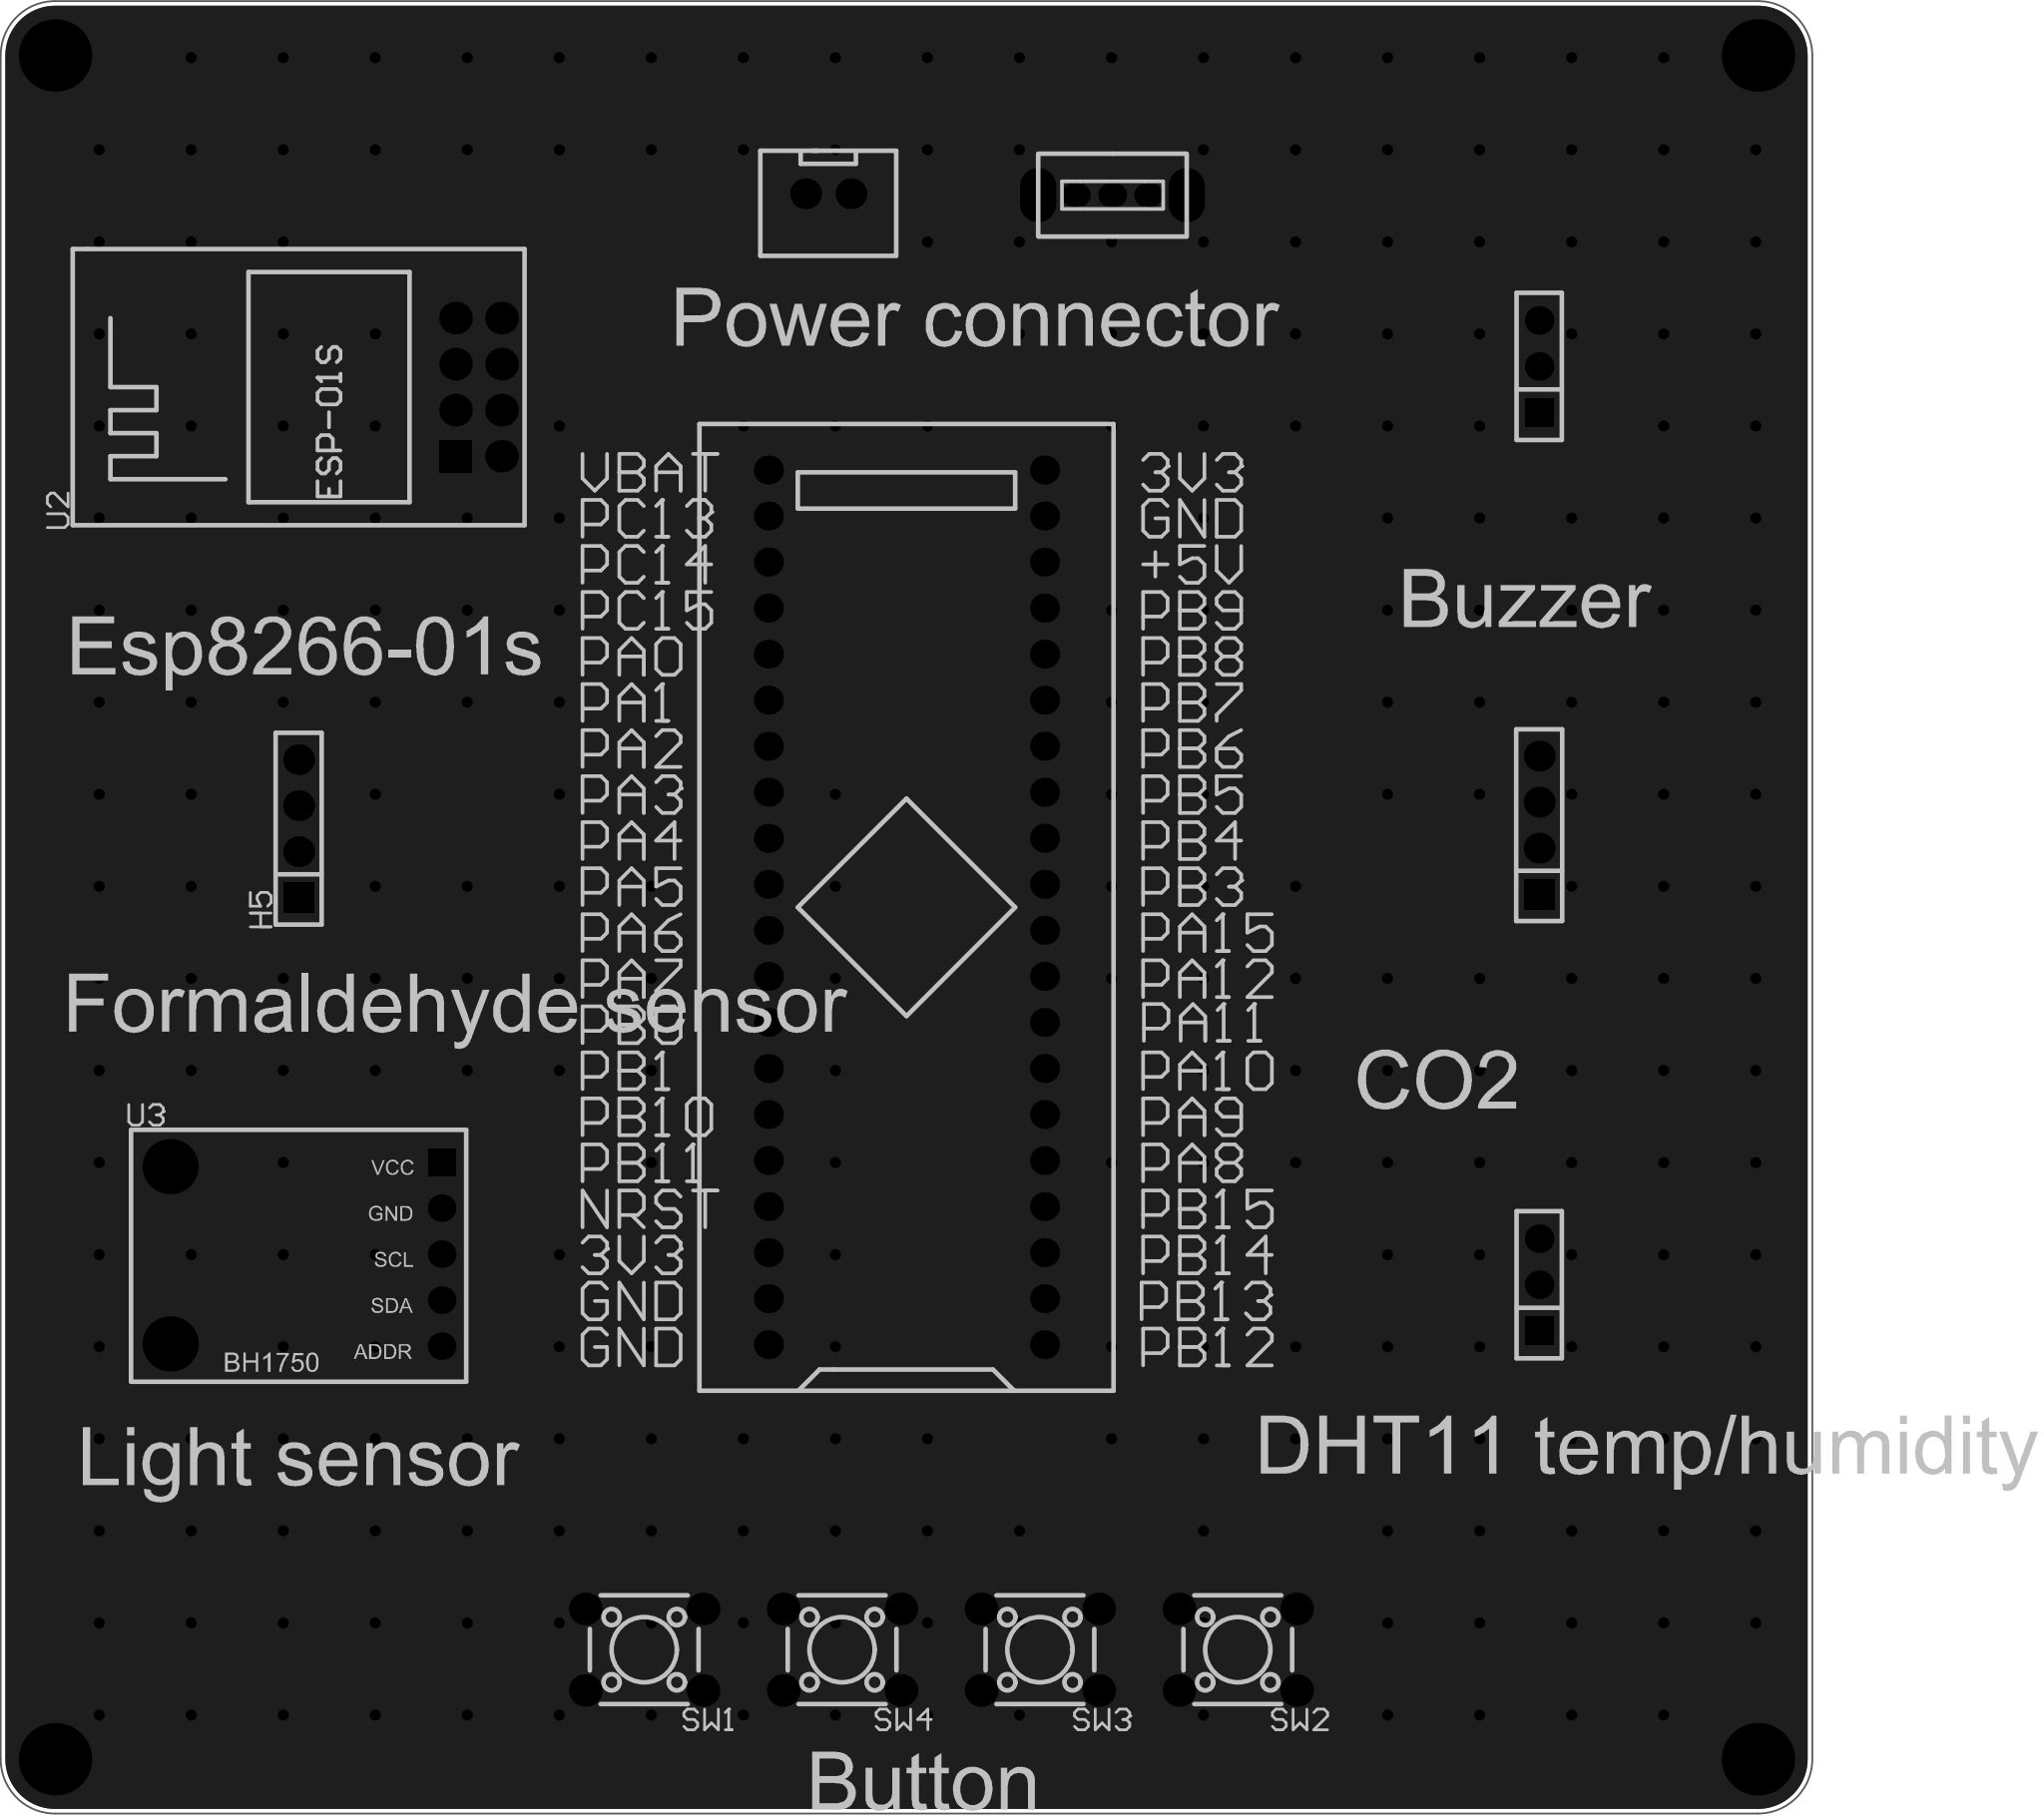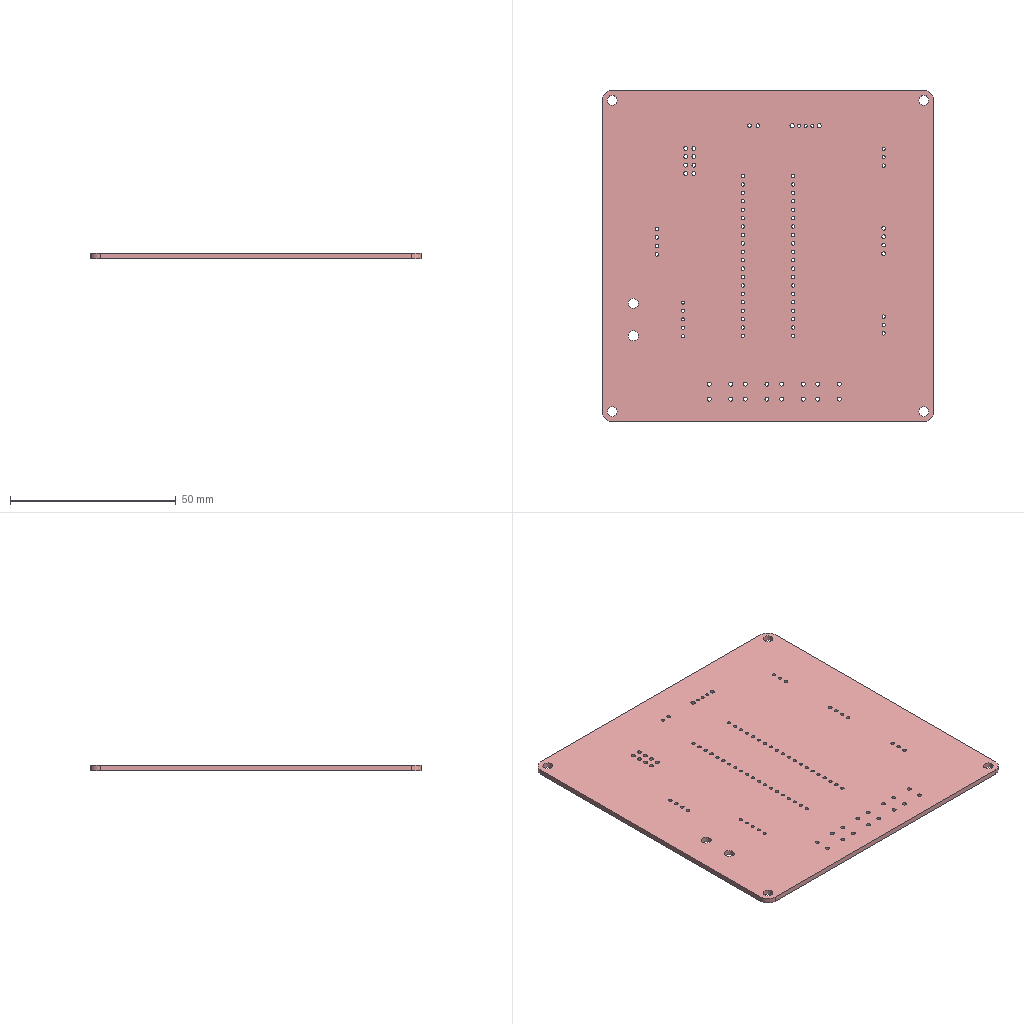Circuit board layout | Altium Designer | box 100 x 100 x 1.6 mm
Layer stack:
# Altium Designer layer stack of  (unit mm; dielectric type: 0 none, 1 core, 2 prepreg, 3 surface material)
index,name,kind,layer,copper_thickness_mm,dielectric_type,dielectric_thickness_mm,dielectric_material,dielectric_constant
0,Top Paste Mask Layer,other,,,,,,
1,Top Silkscreen Layer,other,,,,,,
2,Top Solder Mask Layer,dielectric,,,3,0.01,,3.3
3,Top Layer,copper,Top Layer,0.035,,,,
4,Dielectric1,dielectric,,,3,1.51,FR4,4.5
5,Bottom Layer,copper,Bottom Layer,0.035,,,,
6,Bottom Solder Mask Layer,dielectric,,,3,0.01,,3.3
7,Bottom Silkscreen Layer,other,,,,,,
8,Bottom Paste Mask Layer,other,,,,,,
# drill layer pairs: low layer,high layer
drill_pair,Top Layer,Bottom Layer
Part placement:
Designator,Comment,Layer,Footprint,Center-X(mm),Center-Y(mm),Rotation
U1,STM32F103C8T6-Card,TopLayer,CONN-TH_L53.3-W22.9_STM32F103C8T6-CARD,141.351,130.937,90
SW1,,TopLayer,SW-TH_4P-L6.0-W6.0-P4.50-LS6.5,126.873,89.979,180
SW2,,TopLayer,SW-TH_4P-L6.0-W6.0-P4.50-LS6.5,159.639,89.979,180
SW3,,TopLayer,SW-TH_4P-L6.0-W6.0-P4.50-LS6.5,148.717,89.979,180
SW4,,TopLayer,SW-TH_4P-L6.0-W6.0-P4.50-LS6.5,137.795,89.979,180
CN4,XH2.54*2P_Through-hole,TopLayer,CONN-TH_2P-P2.50-XH2.54-2P,137.033,170.307,0
SW5,,TopLayer,拨动开关,152.72,170.232,180
H1,,TopLayer,HDR-TH_3P-P2.54-V-F,176.276,160.782,90
H3,,TopLayer,HDR-TH_3P-P2.54-V-F,176.276,110.113,90
H4,,TopLayer,HDR-TH_4P-P2.54-V-F,176.276,135.47,90
H5,,TopLayer,HDR-TH_4P-P2.54-V-F,107.798,135.275,90
U2,ESP-01S,TopLayer,WIFIM-TH_ESP-01S,117.729,159.639,90
U3,,TopLayer,BH1750光照传感器,108.2,111.805,0
Pad and via stacks:
# Altium Designer via and pad stacks of  (unit mm). Each distinct definition once, with the count of objects using it.
# via: kind,start_layer,end_layer,hole_mm,diameter_mm,mode(0 simple;1 top-mid-bottom;2 full stack),diameter_per_layer,count,example_net
# pad: kind,layer,hole_mm,hole_type(0 round;1 square;2 slot),plating,top_size,top_shape(1 round;2 rect;3 octagon;9 rounded rect),mid_size,bottom_size,mode,footprint,size_per_layer,count,example
pad,Multi-Layer,3,0,plated,4x4,1,4x4,4x4,0,,,4,1
pad,Multi-Layer,1,0,plated,1.6x1.6,1,1.6x1.6,1.6x1.6,0,CONN-TH_L53.3-W22.9_STM32F103C8T6-CARD,,40,U1.1
pad,Multi-Layer,1.2,0,plated,1.8x1.8,1,1.8x1.8,1.8x1.8,0,SW-TH_4P-L6.0-W6.0-P4.50-LS6.5,,16,SW1.1
pad,Multi-Layer,1.05,0,plated,1.7x1.7,1,1.7x1.7,1.7x1.7,0,CONN-TH_2P-P2.50-XH2.54-2P,,2,CN4.2
pad,Multi-Layer,0.8992,0,plated,1.6x1.3,1,1.6x1.3,1.6x1.3,0,\u00B2\u00A6\u00B6\u00AF\u00BF\u00AA\u00B9\u00D8,,3,SW5.1
pad,Multi-Layer,1.3,0,plated,3x1.999,1,3x1.999,3x1.999,0,\u00B2\u00A6\u00B6\u00AF\u00BF\u00AA\u00B9\u00D8,,2,SW5.4
pad,Multi-Layer,1.02,0,plated,1.575x1.575,1,1.575x1.575,1.575x1.575,0,HDR-TH_3P-P2.54-V-F,,4,H1.3
pad,Multi-Layer,1.02,0,plated,1.575x1.575,2,1.575x1.575,1.575x1.575,0,HDR-TH_3P-P2.54-V-F,,2,H1.1
pad,Multi-Layer,1.1,0,plated,1.7x1.7,2,1.7x1.7,1.7x1.7,0,HDR-TH_4P-P2.54-V-F,,2,H4.1
pad,Multi-Layer,1.1,0,plated,1.7x1.7,1,1.7x1.7,1.7x1.7,0,HDR-TH_4P-P2.54-V-F,,6,H4.2
pad,Multi-Layer,1.2,0,plated,1.8x1.8,2,1.8x1.8,1.8x1.8,0,WIFIM-TH_ESP-01S,,1,U2.1
pad,Multi-Layer,1.2,0,plated,1.8x1.8,1,1.8x1.8,1.8x1.8,0,WIFIM-TH_ESP-01S,,7,U2.2
pad,Multi-Layer,3.048,0,unplated,3.048x3.048,1,3.048x3.048,3.048x3.048,0,BH1750\u00B9\u00E2\u00D5\u00D5\u00B4\u00AB\u00B8\u00D0\u00C6\u00F7,,2,U3.
pad,Multi-Layer,0.9144,0,plated,1.524x1.524,2,1.524x1.524,1.524x1.524,0,BH1750\u00B9\u00E2\u00D5\u00D5\u00B4\u00AB\u00B8\u00D0\u00C6\u00F7,,1,U3.1
pad,Multi-Layer,0.9144,0,plated,1.524x1.524,1,1.524x1.524,1.524x1.524,0,BH1750\u00B9\u00E2\u00D5\u00D5\u00B4\u00AB\u00B8\u00D0\u00C6\u00F7,,4,U3.4
via,Top Layer,Bottom Layer,0.3048,0.61,0,,276,GND
Copper pours:
name,layer,net,type(0 solid;1 hatched;2 none)
Bottom Layer-GND,Bottom Layer,GND,0
Top Layer-GND,Top Layer,GND,0
Design rules, without the lines most boards share:
# Altium Designer design rules of  (exported by Altium Designer, unit mm)
# columns: name | kind | enabled | priority | scope1 | scope2 | descriptor | typed fields (field=value)
Copper_copperRegion_copperThickness1oz | 0 | disabled | 4 | All | All | Clearance Constraint (Gap=5.984mil) (Disabled)(All),(All) | gap=0.152
Copper_copperRegion_copperThickness1oz_1 | 63 | disabled | 4 | All | All | Board Clearance Constraint (Gap=0mil) (Disabled)(All) |
Copper_copperRegion_Copper_copperRegion | 0 | disabled | 5 | All | All | Clearance Constraint (Gap=5.984mil) (Disabled)(All),(All) | gap=0.152
Copper_copperRegion_Copper_copperRegion_1 | 63 | disabled | 5 | All | All | Board Clearance Constraint (Gap=0mil) (Disabled)(All) |
copperThickness1oz | 0 | enabled | 6 | All | All | Clearance Constraint (Gap=5.984mil) (All),(All) | gap=0.152
copperThickness1oz_1 | 63 | enabled | 6 | All | All | Board Clearance Constraint (Gap=0mil) (All) |
copperRegion_copperThickness1oz | 20 | disabled | 1 | All | All | Polygon Connect Rule(Relief Connect )(Conductor Width=10mil) (Relief Angle=90 Angle) (Entries=4) (Air Gap Width=10mil) (Disabled)(All),(All) | connect_style(0=relief,1=direct,2=none)=0 relief_conductor_width=0.254 relief_entries=4
copperRegion_Copper_copperRegion | 20 | disabled | 2 | All | All | Polygon Connect Rule(Relief Connect )(Conductor Width=10mil) (Relief Angle=90 Angle) (Entries=4) (Air Gap Width=10mil) (Disabled)(All),(All) | connect_style(0=relief,1=direct,2=none)=0 relief_conductor_width=0.254 relief_entries=4
copperRegion | 20 | enabled | 3 | All | All | Polygon Connect Rule(Relief Connect )(Conductor Width=10mil) (Relief Angle=90 Angle) (Entries=4) (Air Gap Width=10mil) (All),(All) | connect_style(0=relief,1=direct,2=none)=0 relief_conductor_width=0.254 relief_entries=4